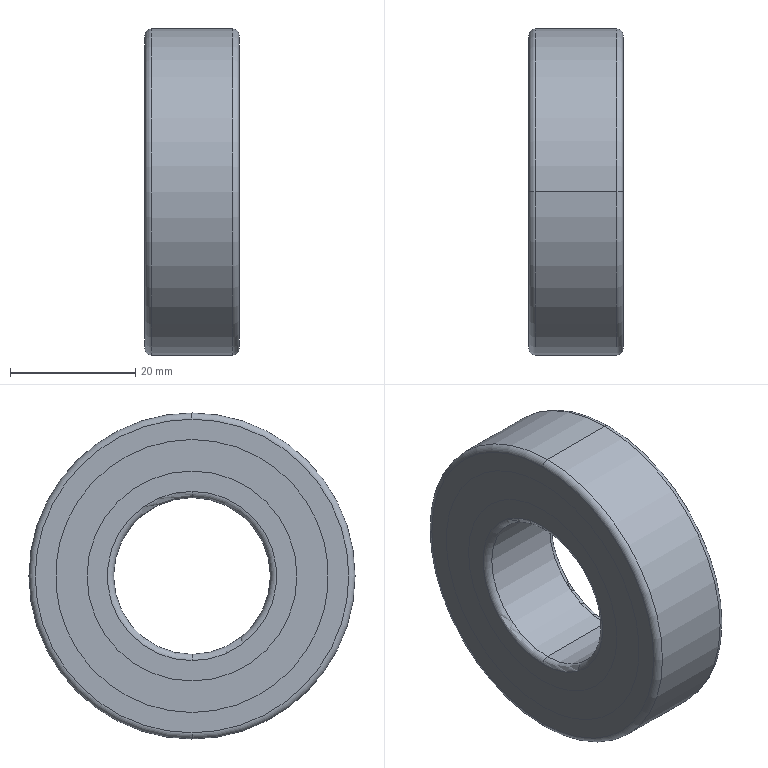Part | STEP file | 6205ZZ_6205ZZ | 5 solids | 46 faces | box 15 x 52 x 52 mm | volume 22330 mm3 | cylinder 20 | torus 18 | plane 8 | commonest cylinder face diameters 33.483 x8 43.517 x8 25 x2 52 x2